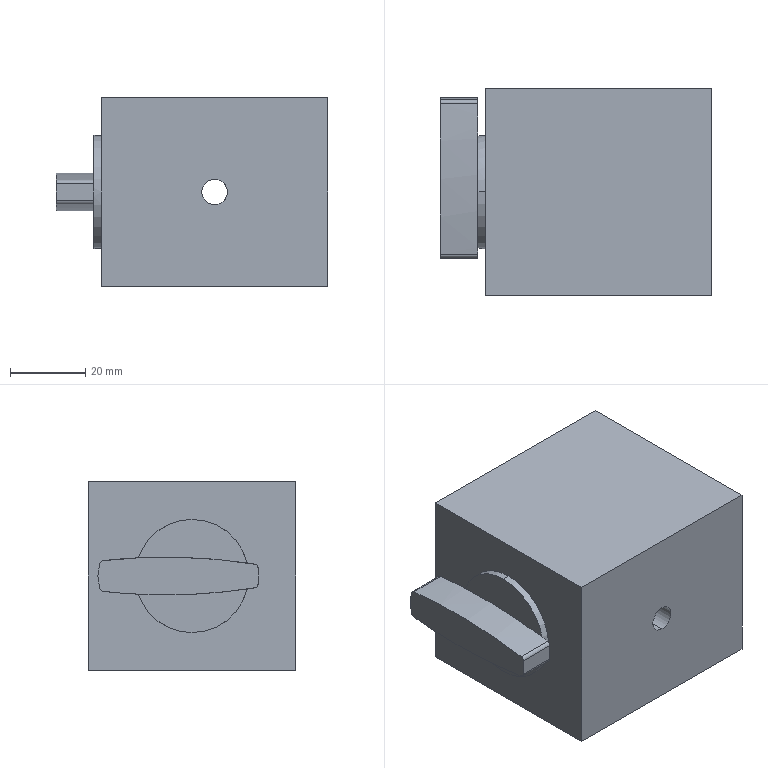Part | SolidWorks | features BaseBody 1 | 1 solid | 28 faces | box 72 x 55 x 50 mm | volume 168174 mm3 | plane 14 | cylinder 12 | cone 2 | commonest cylinder face diameters 2 x5 301.289 x3 6.8 x2 30 x2
STEP:
#1=CARTESIAN_POINT('',(0.,0.,-3.4));
#2=VERTEX_POINT('',#1);
#3=CARTESIAN_POINT('',(0.,0.,3.4));
#4=VERTEX_POINT('',#3);
#5=CARTESIAN_POINT('',(0.,0.,0.));
#6=DIRECTION('',(0.,1.,0.));
#7=DIRECTION('',(0.,0.,1.));
#8=AXIS2_PLACEMENT_3D('',#5,#6,#7);
#9=CIRCLE('',#8,3.4);
#10=EDGE_CURVE('',#2,#4,#9,.T.);
#11=ORIENTED_EDGE('',*,*,#10,.F.);
#12=CARTESIAN_POINT('',(0.,54.375,-3.4));
#13=VERTEX_POINT('',#12);
#14=CARTESIAN_POINT('',(0.,55.,-3.4));
#15=DIRECTION('',(0.,1.,0.));
#16=VECTOR('',#15,1000.);
#17=LINE('',#14,#16);
#18=EDGE_CURVE('',#2,#13,#17,.T.);
#19=ORIENTED_EDGE('',*,*,#18,.T.);
#20=CARTESIAN_POINT('',(-3.4,54.375,0.));
#21=VERTEX_POINT('',#20);
#22=CARTESIAN_POINT('',(0.,54.375,0.));
#23=DIRECTION('',(0.,-1.,0.));
#24=DIRECTION('',(0.,0.,1.));
#25=AXIS2_PLACEMENT_3D('',#22,#23,#24);
#26=CIRCLE('',#25,3.4);
#27=EDGE_CURVE('',#21,#13,#26,.T.);
#28=ORIENTED_EDGE('',*,*,#27,.F.);
#29=CARTESIAN_POINT('',(0.,54.375,3.4));
#30=VERTEX_POINT('',#29);
#31=CARTESIAN_POINT('',(0.,54.375,0.));
#32=DIRECTION('',(0.,-1.,0.));
#33=DIRECTION('',(0.,0.,1.));
#34=AXIS2_PLACEMENT_3D('',#31,#32,#33);
#35=CIRCLE('',#34,3.4);
#36=EDGE_CURVE('',#30,#21,#35,.T.);
#37=ORIENTED_EDGE('',*,*,#36,.F.);
#38=CARTESIAN_POINT('',(0.,55.,3.4));
#39=DIRECTION('',(0.,1.,0.));
#40=VECTOR('',#39,1000.);
#41=LINE('',#38,#40);
#42=EDGE_CURVE('',#4,#30,#41,.T.);
#43=ORIENTED_EDGE('',*,*,#42,.F.);
#44=EDGE_LOOP('',(#11,#19,#28,#37,#43));
#45=FACE_OUTER_BOUND('',#44,.T.);
#46=CARTESIAN_POINT('',(0.,55.,0.));
#47=DIRECTION('',(0.,1.,0.));
#48=DIRECTION('',(0.,0.,1.));
#49=AXIS2_PLACEMENT_3D('',#46,#47,#48);
#50=CYLINDRICAL_SURFACE('',#49,3.4);
#51=ADVANCED_FACE('',(#45),#50,.F.);
#52=ORIENTED_EDGE('',*,*,#27,.T.);
#53=CARTESIAN_POINT('',(3.4,54.375,0.));
#54=VERTEX_POINT('',#53);
#55=CARTESIAN_POINT('',(0.,54.375,0.));
#56=DIRECTION('',(0.,-1.,0.));
#57=DIRECTION('',(0.,0.,1.));
#58=AXIS2_PLACEMENT_3D('',#55,#56,#57);
#59=CIRCLE('',#58,3.4);
#60=EDGE_CURVE('',#13,#54,#59,.T.);
#61=ORIENTED_EDGE('',*,*,#60,.T.);
#62=CARTESIAN_POINT('',(4.025,55.,0.));
#63=VERTEX_POINT('',#62);
#64=CARTESIAN_POINT('',(4.025,55.,0.));
#65=DIRECTION('',(0.7071,0.7071,0.));
#66=VECTOR('',#65,1000.);
#67=LINE('',#64,#66);
#68=EDGE_CURVE('',#54,#63,#67,.T.);
#69=ORIENTED_EDGE('',*,*,#68,.T.);
#70=CARTESIAN_POINT('',(-4.025,55.,0.));
#71=VERTEX_POINT('',#70);
#72=CARTESIAN_POINT('',(0.,55.,0.));
#73=DIRECTION('',(0.,1.,0.));
#74=DIRECTION('',(-1.,0.,0.));
#75=AXIS2_PLACEMENT_3D('',#72,#73,#74);
#76=CIRCLE('',#75,4.025);
#77=EDGE_CURVE('',#63,#71,#76,.T.);
#78=ORIENTED_EDGE('',*,*,#77,.T.);
#79=CARTESIAN_POINT('',(-4.025,55.,0.));
#80=DIRECTION('',(-0.7071,0.7071,0.));
#81=VECTOR('',#80,1000.);
#82=LINE('',#79,#81);
#83=EDGE_CURVE('',#21,#71,#82,.T.);
#84=ORIENTED_EDGE('',*,*,#83,.F.);
#85=EDGE_LOOP('',(#52,#61,#69,#78,#84));
#86=FACE_OUTER_BOUND('',#85,.T.);
#87=CARTESIAN_POINT('',(0.,55.,0.));
#88=DIRECTION('',(0.,1.,0.));
#89=DIRECTION('',(-1.,0.,0.));
#90=AXIS2_PLACEMENT_3D('',#87,#88,#89);
#91=CONICAL_SURFACE('',#90,4.025,0.7854);
#92=ADVANCED_FACE('',(#86),#91,.F.);
#93=CARTESIAN_POINT('',(-32.,41.702,4.826));
#94=VERTEX_POINT('',#93);
#95=CARTESIAN_POINT('',(-32.,27.5,15.));
#96=VERTEX_POINT('',#95);
#97=CARTESIAN_POINT('',(-32.,27.5,0.));
#98=DIRECTION('',(1.,0.,0.));
#99=DIRECTION('',(0.,0.,-1.));
#100=AXIS2_PLACEMENT_3D('',#97,#98,#99);
#101=CIRCLE('',#100,15.);
#102=EDGE_CURVE('',#94,#96,#101,.T.);
#103=ORIENTED_EDGE('',*,*,#102,.T.);
#104=CARTESIAN_POINT('',(-30.,27.5,15.));
#105=VERTEX_POINT('',#104);
#106=CARTESIAN_POINT('',(-32.,27.5,15.));
#107=DIRECTION('',(1.,0.,0.));
#108=VECTOR('',#107,1000.);
#109=LINE('',#106,#108);
#110=EDGE_CURVE('',#96,#105,#109,.T.);
#111=ORIENTED_EDGE('',*,*,#110,.T.);
#112=CARTESIAN_POINT('',(-30.,27.5,-15.));
#113=VERTEX_POINT('',#112);
#114=CARTESIAN_POINT('',(-30.,27.5,0.));
#115=DIRECTION('',(-1.,0.,0.));
#116=DIRECTION('',(0.,0.,-1.));
#117=AXIS2_PLACEMENT_3D('',#114,#115,#116);
#118=CIRCLE('',#117,15.);
#119=EDGE_CURVE('',#105,#113,#118,.T.);
#120=ORIENTED_EDGE('',*,*,#119,.T.);
#121=CARTESIAN_POINT('',(-32.,27.5,-15.));
#122=VERTEX_POINT('',#121);
#123=CARTESIAN_POINT('',(-32.,27.5,-15.));
#124=DIRECTION('',(1.,0.,0.));
#125=VECTOR('',#124,1000.);
#126=LINE('',#123,#125);
#127=EDGE_CURVE('',#122,#113,#126,.T.);
#128=ORIENTED_EDGE('',*,*,#127,.F.);
#129=CARTESIAN_POINT('',(-32.,41.702,-4.826));
#130=VERTEX_POINT('',#129);
#131=CARTESIAN_POINT('',(-32.,27.5,0.));
#132=DIRECTION('',(1.,0.,0.));
#133=DIRECTION('',(0.,0.,-1.));
#134=AXIS2_PLACEMENT_3D('',#131,#132,#133);
#135=CIRCLE('',#134,15.);
#136=EDGE_CURVE('',#122,#130,#135,.T.);
#137=ORIENTED_EDGE('',*,*,#136,.T.);
#138=CARTESIAN_POINT('',(-32.,27.5,0.));
#139=DIRECTION('',(1.,0.,0.));
#140=DIRECTION('',(0.,0.,-1.));
#141=AXIS2_PLACEMENT_3D('',#138,#139,#140);
#142=CIRCLE('',#141,15.);
#143=EDGE_CURVE('',#130,#94,#142,.T.);
#144=ORIENTED_EDGE('',*,*,#143,.T.);
#145=EDGE_LOOP('',(#103,#111,#120,#128,#137,#144));
#146=FACE_OUTER_BOUND('',#145,.T.);
#147=CARTESIAN_POINT('',(-32.,27.5,0.));
#148=DIRECTION('',(1.,0.,0.));
#149=DIRECTION('',(0.,0.,-1.));
#150=AXIS2_PLACEMENT_3D('',#147,#148,#149);
#151=CYLINDRICAL_SURFACE('',#150,15.);
#152=ADVANCED_FACE('',(#146),#151,.T.);
#153=CARTESIAN_POINT('',(-42.,10.843,-3.136));
#154=VERTEX_POINT('',#153);
#155=CARTESIAN_POINT('',(-42.,34.466,-5.));
#156=VERTEX_POINT('',#155);
#157=CARTESIAN_POINT('',(-42.,34.466,145.644));
#158=DIRECTION('',(1.,0.,0.));
#159=DIRECTION('',(0.,0.,-1.));
#160=AXIS2_PLACEMENT_3D('',#157,#158,#159);
#161=CIRCLE('',#160,150.644);
#162=EDGE_CURVE('',#154,#156,#161,.T.);
#163=ORIENTED_EDGE('',*,*,#162,.T.);
#164=CARTESIAN_POINT('',(-32.,34.466,-5.));
#165=VERTEX_POINT('',#164);
#166=CARTESIAN_POINT('',(-42.,34.466,-5.));
#167=DIRECTION('',(1.,0.,0.));
#168=VECTOR('',#167,1000.);
#169=LINE('',#166,#168);
#170=EDGE_CURVE('',#156,#165,#169,.T.);
#171=ORIENTED_EDGE('',*,*,#170,.T.);
#172=CARTESIAN_POINT('',(-32.,12.902,-3.449));
#173=VERTEX_POINT('',#172);
#174=CARTESIAN_POINT('',(-32.,34.466,145.644));
#175=DIRECTION('',(1.,0.,0.));
#176=DIRECTION('',(0.,0.,-1.));
#177=AXIS2_PLACEMENT_3D('',#174,#175,#176);
#178=CIRCLE('',#177,150.644);
#179=EDGE_CURVE('',#173,#165,#178,.T.);
#180=ORIENTED_EDGE('',*,*,#179,.F.);
#181=CARTESIAN_POINT('',(-32.,10.843,-3.136));
#182=VERTEX_POINT('',#181);
#183=CARTESIAN_POINT('',(-32.,34.466,145.644));
#184=DIRECTION('',(1.,0.,0.));
#185=DIRECTION('',(0.,0.,-1.));
#186=AXIS2_PLACEMENT_3D('',#183,#184,#185);
#187=CIRCLE('',#186,150.644);
#188=EDGE_CURVE('',#182,#173,#187,.T.);
#189=ORIENTED_EDGE('',*,*,#188,.F.);
#190=CARTESIAN_POINT('',(-42.,10.843,-3.136));
#191=DIRECTION('',(-1.,0.,0.));
#192=VECTOR('',#191,1000.);
#193=LINE('',#190,#192);
#194=EDGE_CURVE('',#182,#154,#193,.T.);
#195=ORIENTED_EDGE('',*,*,#194,.T.);
#196=EDGE_LOOP('',(#163,#171,#180,#189,#195));
#197=FACE_OUTER_BOUND('',#196,.T.);
#198=CARTESIAN_POINT('',(-42.,34.466,145.644));
#199=DIRECTION('',(1.,0.,0.));
#200=DIRECTION('',(0.,0.,-1.));
#201=AXIS2_PLACEMENT_3D('',#198,#199,#200);
#202=CYLINDRICAL_SURFACE('',#201,150.644);
#203=ADVANCED_FACE('',(#197),#202,.T.);
#204=CARTESIAN_POINT('',(-30.,55.,-25.));
#205=VERTEX_POINT('',#204);
#206=CARTESIAN_POINT('',(-30.,0.,-25.));
#207=VERTEX_POINT('',#206);
#208=CARTESIAN_POINT('',(-30.,55.,-25.));
#209=DIRECTION('',(0.,-1.,0.));
#210=VECTOR('',#209,1000.);
#211=LINE('',#208,#210);
#212=EDGE_CURVE('',#205,#207,#211,.T.);
#213=ORIENTED_EDGE('',*,*,#212,.F.);
#214=CARTESIAN_POINT('',(30.,55.,-25.));
#215=VERTEX_POINT('',#214);
#216=CARTESIAN_POINT('',(-30.,55.,-25.));
#217=DIRECTION('',(-1.,0.,0.));
#218=VECTOR('',#217,1000.);
#219=LINE('',#216,#218);
#220=EDGE_CURVE('',#215,#205,#219,.T.);
#221=ORIENTED_EDGE('',*,*,#220,.F.);
#222=CARTESIAN_POINT('',(30.,0.,-25.));
#223=VERTEX_POINT('',#222);
#224=CARTESIAN_POINT('',(30.,55.,-25.));
#225=DIRECTION('',(0.,1.,0.));
#226=VECTOR('',#225,1000.);
#227=LINE('',#224,#226);
#228=EDGE_CURVE('',#223,#215,#227,.T.);
#229=ORIENTED_EDGE('',*,*,#228,.F.);
#230=CARTESIAN_POINT('',(-30.,0.,-25.));
#231=DIRECTION('',(1.,0.,0.));
#232=VECTOR('',#231,1000.);
#233=LINE('',#230,#232);
#234=EDGE_CURVE('',#207,#223,#233,.T.);
#235=ORIENTED_EDGE('',*,*,#234,.F.);
#236=EDGE_LOOP('',(#213,#221,#229,#235));
#237=FACE_OUTER_BOUND('',#236,.T.);
#238=CARTESIAN_POINT('',(-30.,55.,-25.));
#239=DIRECTION('',(0.,0.,1.));
#240=DIRECTION('',(1.,0.,0.));
#241=AXIS2_PLACEMENT_3D('',#238,#239,#240);
#242=PLANE('',#241);
#243=ADVANCED_FACE('',(#237),#242,.F.);
#244=CARTESIAN_POINT('',(-30.,0.,25.));
#245=VERTEX_POINT('',#244);
#246=CARTESIAN_POINT('',(-30.,0.,0.));
#247=DIRECTION('',(0.,0.,-1.));
#248=VECTOR('',#247,1000.);
#249=LINE('',#246,#248);
#250=EDGE_CURVE('',#245,#207,#249,.T.);
#251=ORIENTED_EDGE('',*,*,#250,.T.);
#252=ORIENTED_EDGE('',*,*,#234,.T.);
#253=CARTESIAN_POINT('',(30.,0.,25.));
#254=VERTEX_POINT('',#253);
#255=CARTESIAN_POINT('',(30.,0.,0.));
#256=DIRECTION('',(0.,0.,1.));
#257=VECTOR('',#256,1000.);
#258=LINE('',#255,#257);
#259=EDGE_CURVE('',#223,#254,#258,.T.);
#260=ORIENTED_EDGE('',*,*,#259,.T.);
#261=CARTESIAN_POINT('',(0.,0.,25.));
#262=DIRECTION('',(-1.,0.,0.));
#263=VECTOR('',#262,1000.);
#264=LINE('',#261,#263);
#265=EDGE_CURVE('',#254,#245,#264,.T.);
#266=ORIENTED_EDGE('',*,*,#265,.T.);
#267=EDGE_LOOP('',(#251,#252,#260,#266));
#268=FACE_OUTER_BOUND('',#267,.T.);
#269=CARTESIAN_POINT('',(0.,0.,0.));
#270=DIRECTION('',(0.,1.,0.));
#271=DIRECTION('',(0.,0.,1.));
#272=AXIS2_PLACEMENT_3D('',#269,#270,#271);
#273=CIRCLE('',#272,3.4);
#274=EDGE_CURVE('',#4,#2,#273,.T.);
#275=ORIENTED_EDGE('',*,*,#274,.T.);
#276=ORIENTED_EDGE('',*,*,#10,.T.);
#277=EDGE_LOOP('',(#275,#276));
#278=FACE_BOUND('',#277,.T.);
#279=CARTESIAN_POINT('',(0.,0.,0.));
#280=DIRECTION('',(0.,-1.,0.));
#281=DIRECTION('',(0.,0.,-1.));
#282=AXIS2_PLACEMENT_3D('',#279,#280,#281);
#283=PLANE('',#282);
#284=ADVANCED_FACE('',(#268,#278),#283,.T.);
#285=CARTESIAN_POINT('',(-30.,27.5,0.));
#286=DIRECTION('',(-1.,0.,0.));
#287=DIRECTION('',(0.,0.,-1.));
#288=AXIS2_PLACEMENT_3D('',#285,#286,#287);
#289=CIRCLE('',#288,15.);
#290=EDGE_CURVE('',#113,#105,#289,.T.);
#291=ORIENTED_EDGE('',*,*,#290,.F.);
#292=ORIENTED_EDGE('',*,*,#119,.F.);
#293=EDGE_LOOP('',(#291,#292));
#294=FACE_BOUND('',#293,.T.);
#295=CARTESIAN_POINT('',(-30.,55.,25.));
#296=VERTEX_POINT('',#295);
#297=CARTESIAN_POINT('',(-30.,55.,25.));
#298=DIRECTION('',(0.,-1.,0.));
#299=VECTOR('',#298,1000.);
#300=LINE('',#297,#299);
#301=EDGE_CURVE('',#296,#245,#300,.T.);
#302=ORIENTED_EDGE('',*,*,#301,.F.);
#303=CARTESIAN_POINT('',(-30.,55.,25.));
#304=DIRECTION('',(0.,0.,1.));
#305=VECTOR('',#304,1000.);
#306=LINE('',#303,#305);
#307=EDGE_CURVE('',#205,#296,#306,.T.);
#308=ORIENTED_EDGE('',*,*,#307,.F.);
#309=ORIENTED_EDGE('',*,*,#212,.T.);
#310=ORIENTED_EDGE('',*,*,#250,.F.);
#311=EDGE_LOOP('',(#302,#308,#309,#310));
#312=FACE_OUTER_BOUND('',#311,.T.);
#313=CARTESIAN_POINT('',(-30.,55.,25.));
#314=DIRECTION('',(1.,0.,0.));
#315=DIRECTION('',(0.,0.,-1.));
#316=AXIS2_PLACEMENT_3D('',#313,#314,#315);
#317=PLANE('',#316);
#318=ADVANCED_FACE('',(#294,#312),#317,.F.);
#319=ORIENTED_EDGE('',*,*,#220,.T.);
#320=ORIENTED_EDGE('',*,*,#307,.T.);
#321=CARTESIAN_POINT('',(30.,55.,25.));
#322=VERTEX_POINT('',#321);
#323=CARTESIAN_POINT('',(0.,55.,25.));
#324=DIRECTION('',(-1.,0.,0.));
#325=VECTOR('',#324,1000.);
#326=LINE('',#323,#325);
#327=EDGE_CURVE('',#322,#296,#326,.T.);
#328=ORIENTED_EDGE('',*,*,#327,.F.);
#329=CARTESIAN_POINT('',(30.,55.,0.));
#330=DIRECTION('',(0.,0.,1.));
#331=VECTOR('',#330,1000.);
#332=LINE('',#329,#331);
#333=EDGE_CURVE('',#215,#322,#332,.T.);
#334=ORIENTED_EDGE('',*,*,#333,.F.);
#335=EDGE_LOOP('',(#319,#320,#328,#334));
#336=FACE_OUTER_BOUND('',#335,.T.);
#337=CARTESIAN_POINT('',(0.,55.,0.));
#338=DIRECTION('',(0.,1.,0.));
#339=DIRECTION('',(-1.,0.,0.));
#340=AXIS2_PLACEMENT_3D('',#337,#338,#339);
#341=CIRCLE('',#340,4.025);
#342=EDGE_CURVE('',#71,#63,#341,.T.);
#343=ORIENTED_EDGE('',*,*,#342,.F.);
#344=ORIENTED_EDGE('',*,*,#77,.F.);
#345=EDGE_LOOP('',(#343,#344));
#346=FACE_BOUND('',#345,.T.);
#347=CARTESIAN_POINT('',(0.,55.,0.));
#348=DIRECTION('',(0.,-1.,0.));
#349=DIRECTION('',(0.,0.,-1.));
#350=AXIS2_PLACEMENT_3D('',#347,#348,#349);
#351=PLANE('',#350);
#352=ADVANCED_FACE('',(#336,#346),#351,.F.);
#353=ORIENTED_EDGE('',*,*,#228,.T.);
#354=ORIENTED_EDGE('',*,*,#333,.T.);
#355=CARTESIAN_POINT('',(30.,55.,25.));
#356=DIRECTION('',(0.,1.,0.));
#357=VECTOR('',#356,1000.);
#358=LINE('',#355,#357);
#359=EDGE_CURVE('',#254,#322,#358,.T.);
#360=ORIENTED_EDGE('',*,*,#359,.F.);
#361=ORIENTED_EDGE('',*,*,#259,.F.);
#362=EDGE_LOOP('',(#353,#354,#360,#361));
#363=FACE_OUTER_BOUND('',#362,.T.);
#364=CARTESIAN_POINT('',(30.,55.,25.));
#365=DIRECTION('',(-1.,0.,0.));
#366=DIRECTION('',(0.,0.,1.));
#367=AXIS2_PLACEMENT_3D('',#364,#365,#366);
#368=PLANE('',#367);
#369=ADVANCED_FACE('',(#363),#368,.F.);
#370=ORIENTED_EDGE('',*,*,#359,.T.);
#371=ORIENTED_EDGE('',*,*,#327,.T.);
#372=ORIENTED_EDGE('',*,*,#301,.T.);
#373=ORIENTED_EDGE('',*,*,#265,.F.);
#374=EDGE_LOOP('',(#370,#371,#372,#373));
#375=FACE_OUTER_BOUND('',#374,.T.);
#376=CARTESIAN_POINT('',(-30.,55.,25.));
#377=DIRECTION('',(0.,0.,-1.));
#378=DIRECTION('',(-1.,0.,0.));
#379=AXIS2_PLACEMENT_3D('',#376,#377,#378);
#380=PLANE('',#379);
#381=ADVANCED_FACE('',(#375),#380,.F.);
#382=ORIENTED_EDGE('',*,*,#18,.F.);
#383=ORIENTED_EDGE('',*,*,#274,.F.);
#384=ORIENTED_EDGE('',*,*,#42,.T.);
#385=CARTESIAN_POINT('',(0.,54.375,0.));
#386=DIRECTION('',(0.,-1.,0.));
#387=DIRECTION('',(0.,0.,1.));
#388=AXIS2_PLACEMENT_3D('',#385,#386,#387);
#389=CIRCLE('',#388,3.4);
#390=EDGE_CURVE('',#54,#30,#389,.T.);
#391=ORIENTED_EDGE('',*,*,#390,.F.);
#392=ORIENTED_EDGE('',*,*,#60,.F.);
#393=EDGE_LOOP('',(#382,#383,#384,#391,#392));
#394=FACE_OUTER_BOUND('',#393,.T.);
#395=CARTESIAN_POINT('',(0.,55.,0.));
#396=DIRECTION('',(0.,1.,0.));
#397=DIRECTION('',(0.,0.,1.));
#398=AXIS2_PLACEMENT_3D('',#395,#396,#397);
#399=CYLINDRICAL_SURFACE('',#398,3.4);
#400=ADVANCED_FACE('',(#394),#399,.F.);
#401=ORIENTED_EDGE('',*,*,#68,.F.);
#402=ORIENTED_EDGE('',*,*,#390,.T.);
#403=ORIENTED_EDGE('',*,*,#36,.T.);
#404=ORIENTED_EDGE('',*,*,#83,.T.);
#405=ORIENTED_EDGE('',*,*,#342,.T.);
#406=EDGE_LOOP('',(#401,#402,#403,#404,#405));
#407=FACE_OUTER_BOUND('',#406,.T.);
#408=CARTESIAN_POINT('',(0.,55.,0.));
#409=DIRECTION('',(0.,1.,0.));
#410=DIRECTION('',(-1.,0.,0.));
#411=AXIS2_PLACEMENT_3D('',#408,#409,#410);
#412=CONICAL_SURFACE('',#411,4.025,0.7854);
#413=ADVANCED_FACE('',(#407),#412,.F.);
#414=ORIENTED_EDGE('',*,*,#110,.F.);
#415=CARTESIAN_POINT('',(-32.,12.902,3.449));
#416=VERTEX_POINT('',#415);
#417=CARTESIAN_POINT('',(-32.,27.5,0.));
#418=DIRECTION('',(1.,0.,0.));
#419=DIRECTION('',(0.,0.,-1.));
#420=AXIS2_PLACEMENT_3D('',#417,#418,#419);
#421=CIRCLE('',#420,15.);
#422=EDGE_CURVE('',#96,#416,#421,.T.);
#423=ORIENTED_EDGE('',*,*,#422,.T.);
#424=CARTESIAN_POINT('',(-32.,27.5,0.));
#425=DIRECTION('',(1.,0.,0.));
#426=DIRECTION('',(0.,0.,-1.));
#427=AXIS2_PLACEMENT_3D('',#424,#425,#426);
#428=CIRCLE('',#427,15.);
#429=EDGE_CURVE('',#416,#173,#428,.T.);
#430=ORIENTED_EDGE('',*,*,#429,.T.);
#431=CARTESIAN_POINT('',(-32.,27.5,0.));
#432=DIRECTION('',(1.,0.,0.));
#433=DIRECTION('',(0.,0.,-1.));
#434=AXIS2_PLACEMENT_3D('',#431,#432,#433);
#435=CIRCLE('',#434,15.);
#436=EDGE_CURVE('',#173,#122,#435,.T.);
#437=ORIENTED_EDGE('',*,*,#436,.T.);
#438=ORIENTED_EDGE('',*,*,#127,.T.);
#439=ORIENTED_EDGE('',*,*,#290,.T.);
#440=EDGE_LOOP('',(#414,#423,#430,#437,#438,#439));
#441=FACE_OUTER_BOUND('',#440,.T.);
#442=CARTESIAN_POINT('',(-32.,27.5,0.));
#443=DIRECTION('',(1.,0.,0.));
#444=DIRECTION('',(0.,0.,-1.));
#445=AXIS2_PLACEMENT_3D('',#442,#443,#444);
#446=CYLINDRICAL_SURFACE('',#445,15.);
#447=ADVANCED_FACE('',(#441),#446,.T.);
#448=CARTESIAN_POINT('',(-32.,51.05,4.084));
#449=VERTEX_POINT('',#448);
#450=CARTESIAN_POINT('',(-32.,34.466,-145.644));
#451=DIRECTION('',(1.,0.,0.));
#452=DIRECTION('',(0.,0.,-1.));
#453=AXIS2_PLACEMENT_3D('',#450,#451,#452);
#454=CIRCLE('',#453,150.644);
#455=EDGE_CURVE('',#449,#94,#454,.T.);
#456=ORIENTED_EDGE('',*,*,#455,.T.);
#457=ORIENTED_EDGE('',*,*,#143,.F.);
#458=CARTESIAN_POINT('',(-32.,51.05,-4.084));
#459=VERTEX_POINT('',#458);
#460=CARTESIAN_POINT('',(-32.,34.466,145.644));
#461=DIRECTION('',(1.,0.,0.));
#462=DIRECTION('',(0.,0.,-1.));
#463=AXIS2_PLACEMENT_3D('',#460,#461,#462);
#464=CIRCLE('',#463,150.644);
#465=EDGE_CURVE('',#130,#459,#464,.T.);
#466=ORIENTED_EDGE('',*,*,#465,.T.);
#467=CARTESIAN_POINT('',(-32.,51.924,-3.264));
#468=VERTEX_POINT('',#467);
#469=CARTESIAN_POINT('',(-32.,50.94,-3.09));
#470=DIRECTION('',(-1.,0.,0.));
#471=DIRECTION('',(0.,0.,-1.));
#472=AXIS2_PLACEMENT_3D('',#469,#470,#471);
#473=CIRCLE('',#472,1.);
#474=EDGE_CURVE('',#468,#459,#473,.T.);
#475=ORIENTED_EDGE('',*,*,#474,.F.);
#476=CARTESIAN_POINT('',(-32.,52.469,-0.1736));
#477=VERTEX_POINT('',#476);
#478=CARTESIAN_POINT('',(-32.,51.924,-3.264));
#479=DIRECTION('',(0.,0.1736,0.9848));
#480=VECTOR('',#479,1000.);
#481=LINE('',#478,#480);
#482=EDGE_CURVE('',#468,#477,#481,.T.);
#483=ORIENTED_EDGE('',*,*,#482,.T.);
#484=CARTESIAN_POINT('',(-32.,52.469,0.1736));
#485=VERTEX_POINT('',#484);
#486=CARTESIAN_POINT('',(-32.,51.485,0.));
#487=DIRECTION('',(-1.,0.,0.));
#488=DIRECTION('',(0.,0.,-1.));
#489=AXIS2_PLACEMENT_3D('',#486,#487,#488);
#490=CIRCLE('',#489,1.);
#491=EDGE_CURVE('',#485,#477,#490,.T.);
#492=ORIENTED_EDGE('',*,*,#491,.F.);
#493=CARTESIAN_POINT('',(-32.,51.924,3.264));
#494=VERTEX_POINT('',#493);
#495=CARTESIAN_POINT('',(-32.,52.469,0.1736));
#496=DIRECTION('',(0.,-0.1736,0.9848));
#497=VECTOR('',#496,1000.);
#498=LINE('',#495,#497);
#499=EDGE_CURVE('',#485,#494,#498,.T.);
#500=ORIENTED_EDGE('',*,*,#499,.T.);
#501=CARTESIAN_POINT('',(-32.,50.94,3.09));
#502=DIRECTION('',(-1.,0.,0.));
#503=DIRECTION('',(0.,0.,-1.));
#504=AXIS2_PLACEMENT_3D('',#501,#502,#503);
#505=CIRCLE('',#504,1.);
#506=EDGE_CURVE('',#449,#494,#505,.T.);
#507=ORIENTED_EDGE('',*,*,#506,.F.);
#508=EDGE_LOOP('',(#456,#457,#466,#475,#483,#492,#500,#507));
#509=FACE_OUTER_BOUND('',#508,.T.);
#510=CARTESIAN_POINT('',(-32.,34.466,-145.644));
#511=DIRECTION('',(1.,0.,0.));
#512=DIRECTION('',(0.,0.,-1.));
#513=AXIS2_PLACEMENT_3D('',#510,#511,#512);
#514=PLANE('',#513);
#515=ADVANCED_FACE('',(#509),#514,.T.);
#516=ORIENTED_EDGE('',*,*,#436,.F.);
#517=ORIENTED_EDGE('',*,*,#179,.T.);
#518=CARTESIAN_POINT('',(-32.,34.466,145.644));
#519=DIRECTION('',(1.,0.,0.));
#520=DIRECTION('',(0.,0.,-1.));
#521=AXIS2_PLACEMENT_3D('',#518,#519,#520);
#522=CIRCLE('',#521,150.644);
#523=EDGE_CURVE('',#165,#130,#522,.T.);
#524=ORIENTED_EDGE('',*,*,#523,.T.);
#525=ORIENTED_EDGE('',*,*,#136,.F.);
#526=EDGE_LOOP('',(#516,#517,#524,#525));
#527=FACE_OUTER_BOUND('',#526,.T.);
#528=CARTESIAN_POINT('',(-32.,27.5,0.));
#529=DIRECTION('',(-1.,0.,0.));
#530=DIRECTION('',(0.,0.,1.));
#531=AXIS2_PLACEMENT_3D('',#528,#529,#530);
#532=PLANE('',#531);
#533=ADVANCED_FACE('',(#527),#532,.T.);
#534=CARTESIAN_POINT('',(-32.,34.466,-145.644));
#535=DIRECTION('',(1.,0.,0.));
#536=DIRECTION('',(0.,0.,-1.));
#537=AXIS2_PLACEMENT_3D('',#534,#535,#536);
#538=CIRCLE('',#537,150.644);
#539=EDGE_CURVE('',#94,#416,#538,.T.);
#540=ORIENTED_EDGE('',*,*,#539,.T.);
#541=ORIENTED_EDGE('',*,*,#422,.F.);
#542=ORIENTED_EDGE('',*,*,#102,.F.);
#543=EDGE_LOOP('',(#540,#541,#542));
#544=FACE_OUTER_BOUND('',#543,.T.);
#545=CARTESIAN_POINT('',(-32.,27.5,0.));
#546=DIRECTION('',(-1.,0.,0.));
#547=DIRECTION('',(0.,0.,1.));
#548=AXIS2_PLACEMENT_3D('',#545,#546,#547);
#549=PLANE('',#548);
#550=ADVANCED_FACE('',(#544),#549,.T.);
#551=ORIENTED_EDGE('',*,*,#188,.T.);
#552=ORIENTED_EDGE('',*,*,#429,.F.);
#553=CARTESIAN_POINT('',(-32.,10.843,3.136));
#554=VERTEX_POINT('',#553);
#555=CARTESIAN_POINT('',(-32.,34.466,-145.644));
#556=DIRECTION('',(1.,0.,0.));
#557=DIRECTION('',(0.,0.,-1.));
#558=AXIS2_PLACEMENT_3D('',#555,#556,#557);
#559=CIRCLE('',#558,150.644);
#560=EDGE_CURVE('',#416,#554,#559,.T.);
#561=ORIENTED_EDGE('',*,*,#560,.T.);
#562=CARTESIAN_POINT('',(-32.,10.,2.149));
#563=VERTEX_POINT('',#562);
#564=CARTESIAN_POINT('',(-32.,11.,2.149));
#565=DIRECTION('',(-1.,0.,0.));
#566=DIRECTION('',(0.,0.,-1.));
#567=AXIS2_PLACEMENT_3D('',#564,#565,#566);
#568=CIRCLE('',#567,1.);
#569=EDGE_CURVE('',#563,#554,#568,.T.);
#570=ORIENTED_EDGE('',*,*,#569,.F.);
#571=CARTESIAN_POINT('',(-32.,10.,-2.149));
#572=VERTEX_POINT('',#571);
#573=CARTESIAN_POINT('',(-32.,10.,-145.644));
#574=DIRECTION('',(0.,0.,-1.));
#575=VECTOR('',#574,1000.);
#576=LINE('',#573,#575);
#577=EDGE_CURVE('',#563,#572,#576,.T.);
#578=ORIENTED_EDGE('',*,*,#577,.T.);
#579=CARTESIAN_POINT('',(-32.,11.,-2.149));
#580=DIRECTION('',(-1.,0.,0.));
#581=DIRECTION('',(0.,0.,-1.));
#582=AXIS2_PLACEMENT_3D('',#579,#580,#581);
#583=CIRCLE('',#582,1.);
#584=EDGE_CURVE('',#182,#572,#583,.T.);
#585=ORIENTED_EDGE('',*,*,#584,.F.);
#586=EDGE_LOOP('',(#551,#552,#561,#570,#578,#585));
#587=FACE_OUTER_BOUND('',#586,.T.);
#588=CARTESIAN_POINT('',(-32.,34.466,-145.644));
#589=DIRECTION('',(1.,0.,0.));
#590=DIRECTION('',(0.,0.,-1.));
#591=AXIS2_PLACEMENT_3D('',#588,#589,#590);
#592=PLANE('',#591);
#593=ADVANCED_FACE('',(#587),#592,.T.);
#594=ORIENTED_EDGE('',*,*,#455,.F.);
#595=CARTESIAN_POINT('',(-42.,51.05,4.084));
#596=VERTEX_POINT('',#595);
#597=CARTESIAN_POINT('',(-42.,51.05,4.084));
#598=DIRECTION('',(-1.,0.,0.));
#599=VECTOR('',#598,1000.);
#600=LINE('',#597,#599);
#601=EDGE_CURVE('',#449,#596,#600,.T.);
#602=ORIENTED_EDGE('',*,*,#601,.T.);
#603=CARTESIAN_POINT('',(-42.,10.843,3.136));
#604=VERTEX_POINT('',#603);
#605=CARTESIAN_POINT('',(-42.,34.466,-145.644));
#606=DIRECTION('',(1.,0.,0.));
#607=DIRECTION('',(0.,0.,-1.));
#608=AXIS2_PLACEMENT_3D('',#605,#606,#607);
#609=CIRCLE('',#608,150.644);
#610=EDGE_CURVE('',#596,#604,#609,.T.);
#611=ORIENTED_EDGE('',*,*,#610,.T.);
#612=CARTESIAN_POINT('',(-42.,10.843,3.136));
#613=DIRECTION('',(1.,0.,0.));
#614=VECTOR('',#613,1000.);
#615=LINE('',#612,#614);
#616=EDGE_CURVE('',#604,#554,#615,.T.);
#617=ORIENTED_EDGE('',*,*,#616,.T.);
#618=ORIENTED_EDGE('',*,*,#560,.F.);
#619=ORIENTED_EDGE('',*,*,#539,.F.);
#620=EDGE_LOOP('',(#594,#602,#611,#617,#618,#619));
#621=FACE_OUTER_BOUND('',#620,.T.);
#622=CARTESIAN_POINT('',(-42.,34.466,-145.644));
#623=DIRECTION('',(1.,0.,0.));
#624=DIRECTION('',(0.,0.,-1.));
#625=AXIS2_PLACEMENT_3D('',#622,#623,#624);
#626=CYLINDRICAL_SURFACE('',#625,150.644);
#627=ADVANCED_FACE('',(#621),#626,.T.);
#628=CARTESIAN_POINT('',(-42.,52.469,0.1736));
#629=VERTEX_POINT('',#628);
#630=CARTESIAN_POINT('',(-42.,52.469,0.1736));
#631=DIRECTION('',(1.,0.,0.));
#632=VECTOR('',#631,1000.);
#633=LINE('',#630,#632);
#634=EDGE_CURVE('',#629,#485,#633,.T.);
#635=ORIENTED_EDGE('',*,*,#634,.F.);
#636=CARTESIAN_POINT('',(-42.,51.924,3.264));
#637=VERTEX_POINT('',#636);
#638=CARTESIAN_POINT('',(-42.,52.5,0.));
#639=DIRECTION('',(0.,0.1736,-0.9848));
#640=VECTOR('',#639,1000.);
#641=LINE('',#638,#640);
#642=EDGE_CURVE('',#637,#629,#641,.T.);
#643=ORIENTED_EDGE('',*,*,#642,.F.);
#644=CARTESIAN_POINT('',(-42.,51.924,3.264));
#645=DIRECTION('',(-1.,0.,0.));
#646=VECTOR('',#645,1000.);
#647=LINE('',#644,#646);
#648=EDGE_CURVE('',#494,#637,#647,.T.);
#649=ORIENTED_EDGE('',*,*,#648,.F.);
#650=ORIENTED_EDGE('',*,*,#499,.F.);
#651=EDGE_LOOP('',(#635,#643,#649,#650));
#652=FACE_OUTER_BOUND('',#651,.T.);
#653=CARTESIAN_POINT('',(-42.,52.5,0.));
#654=DIRECTION('',(0.,-0.9848,-0.1736));
#655=DIRECTION('',(0.,0.1736,-0.9848));
#656=AXIS2_PLACEMENT_3D('',#653,#654,#655);
#657=PLANE('',#656);
#658=ADVANCED_FACE('',(#652),#657,.F.);
#659=CARTESIAN_POINT('',(-42.,51.924,-3.264));
#660=VERTEX_POINT('',#659);
#661=CARTESIAN_POINT('',(-42.,51.924,-3.264));
#662=DIRECTION('',(1.,0.,0.));
#663=VECTOR('',#662,1000.);
#664=LINE('',#661,#663);
#665=EDGE_CURVE('',#660,#468,#664,.T.);
#666=ORIENTED_EDGE('',*,*,#665,.F.);
#667=CARTESIAN_POINT('',(-42.,52.469,-0.1736));
#668=VERTEX_POINT('',#667);
#669=CARTESIAN_POINT('',(-42.,52.5,0.));
#670=DIRECTION('',(0.,-0.1736,-0.9848));
#671=VECTOR('',#670,1000.);
#672=LINE('',#669,#671);
#673=EDGE_CURVE('',#668,#660,#672,.T.);
#674=ORIENTED_EDGE('',*,*,#673,.F.);
#675=CARTESIAN_POINT('',(-42.,52.469,-0.1736));
#676=DIRECTION('',(-1.,0.,0.));
#677=VECTOR('',#676,1000.);
#678=LINE('',#675,#677);
#679=EDGE_CURVE('',#477,#668,#678,.T.);
#680=ORIENTED_EDGE('',*,*,#679,.F.);
#681=ORIENTED_EDGE('',*,*,#482,.F.);
#682=EDGE_LOOP('',(#666,#674,#680,#681));
#683=FACE_OUTER_BOUND('',#682,.T.);
#684=CARTESIAN_POINT('',(-42.,52.5,0.));
#685=DIRECTION('',(0.,-0.9848,0.1736));
#686=DIRECTION('',(0.,-0.1736,-0.9848));
#687=AXIS2_PLACEMENT_3D('',#684,#685,#686);
#688=PLANE('',#687);
#689=ADVANCED_FACE('',(#683),#688,.F.);
#690=ORIENTED_EDGE('',*,*,#170,.F.);
#691=CARTESIAN_POINT('',(-42.,51.05,-4.084));
#692=VERTEX_POINT('',#691);
#693=CARTESIAN_POINT('',(-42.,34.466,145.644));
#694=DIRECTION('',(1.,0.,0.));
#695=DIRECTION('',(0.,0.,-1.));
#696=AXIS2_PLACEMENT_3D('',#693,#694,#695);
#697=CIRCLE('',#696,150.644);
#698=EDGE_CURVE('',#156,#692,#697,.T.);
#699=ORIENTED_EDGE('',*,*,#698,.T.);
#700=CARTESIAN_POINT('',(-42.,51.05,-4.084));
#701=DIRECTION('',(1.,0.,0.));
#702=VECTOR('',#701,1000.);
#703=LINE('',#700,#702);
#704=EDGE_CURVE('',#692,#459,#703,.T.);
#705=ORIENTED_EDGE('',*,*,#704,.T.);
#706=ORIENTED_EDGE('',*,*,#465,.F.);
#707=ORIENTED_EDGE('',*,*,#523,.F.);
#708=EDGE_LOOP('',(#690,#699,#705,#706,#707));
#709=FACE_OUTER_BOUND('',#708,.T.);
#710=CARTESIAN_POINT('',(-42.,34.466,145.644));
#711=DIRECTION('',(1.,0.,0.));
#712=DIRECTION('',(0.,0.,-1.));
#713=AXIS2_PLACEMENT_3D('',#710,#711,#712);
#714=CYLINDRICAL_SURFACE('',#713,150.644);
#715=ADVANCED_FACE('',(#709),#714,.T.);
#716=CARTESIAN_POINT('',(-42.,10.,2.149));
#717=VERTEX_POINT('',#716);
#718=CARTESIAN_POINT('',(-42.,10.,2.149));
#719=DIRECTION('',(1.,0.,0.));
#720=VECTOR('',#719,1000.);
#721=LINE('',#718,#720);
#722=EDGE_CURVE('',#717,#563,#721,.T.);
#723=ORIENTED_EDGE('',*,*,#722,.F.);
#724=CARTESIAN_POINT('',(-42.,10.,-2.149));
#725=VERTEX_POINT('',#724);
#726=CARTESIAN_POINT('',(-42.,10.,-3.));
#727=DIRECTION('',(0.,0.,1.));
#728=VECTOR('',#727,1000.);
#729=LINE('',#726,#728);
#730=EDGE_CURVE('',#725,#717,#729,.T.);
#731=ORIENTED_EDGE('',*,*,#730,.F.);
#732=CARTESIAN_POINT('',(-42.,10.,-2.149));
#733=DIRECTION('',(-1.,0.,0.));
#734=VECTOR('',#733,1000.);
#735=LINE('',#732,#734);
#736=EDGE_CURVE('',#572,#725,#735,.T.);
#737=ORIENTED_EDGE('',*,*,#736,.F.);
#738=ORIENTED_EDGE('',*,*,#577,.F.);
#739=EDGE_LOOP('',(#723,#731,#737,#738));
#740=FACE_OUTER_BOUND('',#739,.T.);
#741=CARTESIAN_POINT('',(-42.,10.,-3.));
#742=DIRECTION('',(0.,1.,0.));
#743=DIRECTION('',(0.,0.,1.));
#744=AXIS2_PLACEMENT_3D('',#741,#742,#743);
#745=PLANE('',#744);
#746=ADVANCED_FACE('',(#740),#745,.F.);
#747=ORIENTED_EDGE('',*,*,#506,.T.);
#748=ORIENTED_EDGE('',*,*,#648,.T.);
#749=CARTESIAN_POINT('',(-42.,50.94,3.09));
#750=DIRECTION('',(1.,0.,0.));
#751=DIRECTION('',(0.,0.,-1.));
#752=AXIS2_PLACEMENT_3D('',#749,#750,#751);
#753=CIRCLE('',#752,1.);
#754=EDGE_CURVE('',#637,#596,#753,.T.);
#755=ORIENTED_EDGE('',*,*,#754,.T.);
#756=ORIENTED_EDGE('',*,*,#601,.F.);
#757=EDGE_LOOP('',(#747,#748,#755,#756));
#758=FACE_OUTER_BOUND('',#757,.T.);
#759=CARTESIAN_POINT('',(-42.,50.94,3.09));
#760=DIRECTION('',(1.,0.,0.));
#761=DIRECTION('',(0.,0.,-1.));
#762=AXIS2_PLACEMENT_3D('',#759,#760,#761);
#763=CYLINDRICAL_SURFACE('',#762,1.);
#764=ADVANCED_FACE('',(#758),#763,.T.);
#765=ORIENTED_EDGE('',*,*,#569,.T.);
#766=ORIENTED_EDGE('',*,*,#616,.F.);
#767=CARTESIAN_POINT('',(-42.,11.,2.149));
#768=DIRECTION('',(1.,0.,0.));
#769=DIRECTION('',(0.,0.,-1.));
#770=AXIS2_PLACEMENT_3D('',#767,#768,#769);
#771=CIRCLE('',#770,1.);
#772=EDGE_CURVE('',#604,#717,#771,.T.);
#773=ORIENTED_EDGE('',*,*,#772,.T.);
#774=ORIENTED_EDGE('',*,*,#722,.T.);
#775=EDGE_LOOP('',(#765,#766,#773,#774));
#776=FACE_OUTER_BOUND('',#775,.T.);
#777=CARTESIAN_POINT('',(-42.,11.,2.149));
#778=DIRECTION('',(1.,0.,0.));
#779=DIRECTION('',(0.,0.,-1.));
#780=AXIS2_PLACEMENT_3D('',#777,#778,#779);
#781=CYLINDRICAL_SURFACE('',#780,1.);
#782=ADVANCED_FACE('',(#776),#781,.T.);
#783=ORIENTED_EDGE('',*,*,#772,.F.);
#784=ORIENTED_EDGE('',*,*,#610,.F.);
#785=ORIENTED_EDGE('',*,*,#754,.F.);
#786=ORIENTED_EDGE('',*,*,#642,.T.);
#787=CARTESIAN_POINT('',(-42.,51.485,0.));
#788=DIRECTION('',(1.,0.,0.));
#789=DIRECTION('',(0.,0.,-1.));
#790=AXIS2_PLACEMENT_3D('',#787,#788,#789);
#791=CIRCLE('',#790,1.);
#792=EDGE_CURVE('',#668,#629,#791,.T.);
#793=ORIENTED_EDGE('',*,*,#792,.F.);
#794=ORIENTED_EDGE('',*,*,#673,.T.);
#795=CARTESIAN_POINT('',(-42.,50.94,-3.09));
#796=DIRECTION('',(1.,0.,0.));
#797=DIRECTION('',(0.,0.,-1.));
#798=AXIS2_PLACEMENT_3D('',#795,#796,#797);
#799=CIRCLE('',#798,1.);
#800=EDGE_CURVE('',#692,#660,#799,.T.);
#801=ORIENTED_EDGE('',*,*,#800,.F.);
#802=ORIENTED_EDGE('',*,*,#698,.F.);
#803=ORIENTED_EDGE('',*,*,#162,.F.);
#804=CARTESIAN_POINT('',(-42.,11.,-2.149));
#805=DIRECTION('',(1.,0.,0.));
#806=DIRECTION('',(0.,0.,-1.));
#807=AXIS2_PLACEMENT_3D('',#804,#805,#806);
#808=CIRCLE('',#807,1.);
#809=EDGE_CURVE('',#725,#154,#808,.T.);
#810=ORIENTED_EDGE('',*,*,#809,.F.);
#811=ORIENTED_EDGE('',*,*,#730,.T.);
#812=EDGE_LOOP('',(#783,#784,#785,#786,#793,#794,#801,#802,#803,#810,#811));
#813=FACE_OUTER_BOUND('',#812,.T.);
#814=CARTESIAN_POINT('',(-42.,34.466,-145.644));
#815=DIRECTION('',(1.,0.,0.));
#816=DIRECTION('',(0.,0.,-1.));
#817=AXIS2_PLACEMENT_3D('',#814,#815,#816);
#818=PLANE('',#817);
#819=ADVANCED_FACE('',(#813),#818,.F.);
#820=ORIENTED_EDGE('',*,*,#491,.T.);
#821=ORIENTED_EDGE('',*,*,#679,.T.);
#822=ORIENTED_EDGE('',*,*,#792,.T.);
#823=ORIENTED_EDGE('',*,*,#634,.T.);
#824=EDGE_LOOP('',(#820,#821,#822,#823));
#825=FACE_OUTER_BOUND('',#824,.T.);
#826=CARTESIAN_POINT('',(-42.,51.485,0.));
#827=DIRECTION('',(1.,0.,0.));
#828=DIRECTION('',(0.,0.,-1.));
#829=AXIS2_PLACEMENT_3D('',#826,#827,#828);
#830=CYLINDRICAL_SURFACE('',#829,1.);
#831=ADVANCED_FACE('',(#825),#830,.T.);
#832=ORIENTED_EDGE('',*,*,#474,.T.);
#833=ORIENTED_EDGE('',*,*,#704,.F.);
#834=ORIENTED_EDGE('',*,*,#800,.T.);
#835=ORIENTED_EDGE('',*,*,#665,.T.);
#836=EDGE_LOOP('',(#832,#833,#834,#835));
#837=FACE_OUTER_BOUND('',#836,.T.);
#838=CARTESIAN_POINT('',(-42.,50.94,-3.09));
#839=DIRECTION('',(1.,0.,0.));
#840=DIRECTION('',(0.,0.,-1.));
#841=AXIS2_PLACEMENT_3D('',#838,#839,#840);
#842=CYLINDRICAL_SURFACE('',#841,1.);
#843=ADVANCED_FACE('',(#837),#842,.T.);
#844=ORIENTED_EDGE('',*,*,#584,.T.);
#845=ORIENTED_EDGE('',*,*,#736,.T.);
#846=ORIENTED_EDGE('',*,*,#809,.T.);
#847=ORIENTED_EDGE('',*,*,#194,.F.);
#848=EDGE_LOOP('',(#844,#845,#846,#847));
#849=FACE_OUTER_BOUND('',#848,.T.);
#850=CARTESIAN_POINT('',(-42.,11.,-2.149));
#851=DIRECTION('',(1.,0.,0.));
#852=DIRECTION('',(0.,0.,-1.));
#853=AXIS2_PLACEMENT_3D('',#850,#851,#852);
#854=CYLINDRICAL_SURFACE('',#853,1.);
#855=ADVANCED_FACE('',(#849),#854,.T.);
#856=CLOSED_SHELL('',(#51,#92,#152,#203,#243,#284,#318,#352,#369,#381,#400,#413,#447,#515,#533,#550,#593,#627,#658,#689,#715,#746,#764,#782,#819,#831,#843,#855));
#857=MANIFOLD_SOLID_BREP('',#856);
#858=CARTESIAN_POINT('',(0.,0.,0.));
#859=DIRECTION('',(0.,0.,1.));
#860=DIRECTION('',(1.,0.,0.));
#861=AXIS2_PLACEMENT_3D('',#858,#859,#860);
#862=(LENGTH_UNIT()NAMED_UNIT(*)SI_UNIT(.MILLI.,.METRE.));
#863=UNCERTAINTY_MEASURE_WITH_UNIT(LENGTH_MEASURE(0.00001),#862,'','');
#864=(NAMED_UNIT(*)PLANE_ANGLE_UNIT()SI_UNIT($,.RADIAN.));
#865=(NAMED_UNIT(*)SI_UNIT($,.STERADIAN.)SOLID_ANGLE_UNIT());
#866=(GEOMETRIC_REPRESENTATION_CONTEXT(3)GLOBAL_UNCERTAINTY_ASSIGNED_CONTEXT((#863))GLOBAL_UNIT_ASSIGNED_CONTEXT((#862,#864,#865))REPRESENTATION_CONTEXT('',''));
#867=ADVANCED_BREP_SHAPE_REPRESENTATION('',(#857,#861),#866);